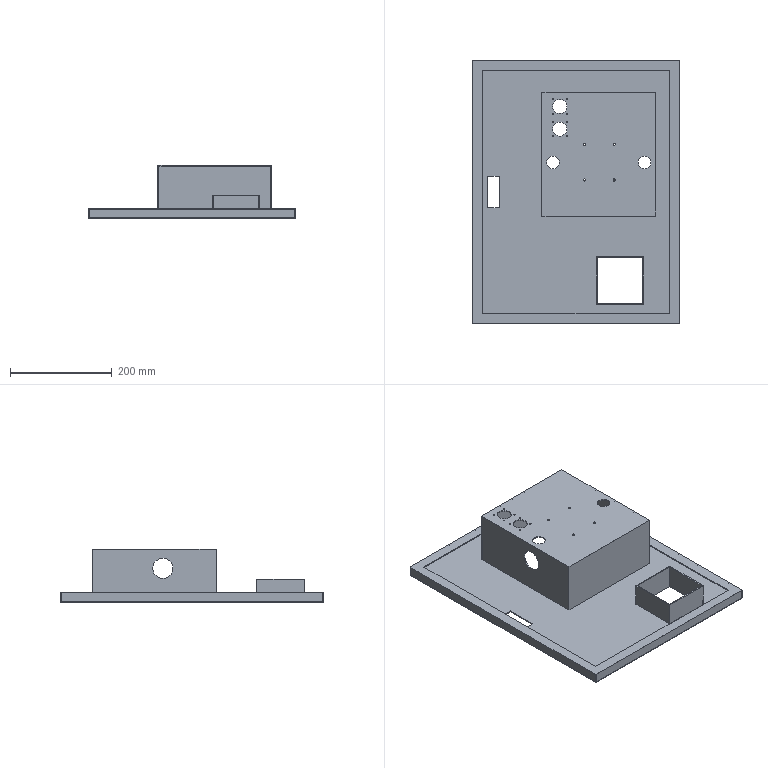Part | STEP file | 11-FG-JX00411 | 1 solid | 87 faces | box 408 x 519 x 106 mm | volume 749356 mm3 | cylinder 44 | plane 39 | sphere 4 | commonest cylinder face diameters 2.5 x16 4 x8 4.2 x8 25 x4 28 x4 40 x4